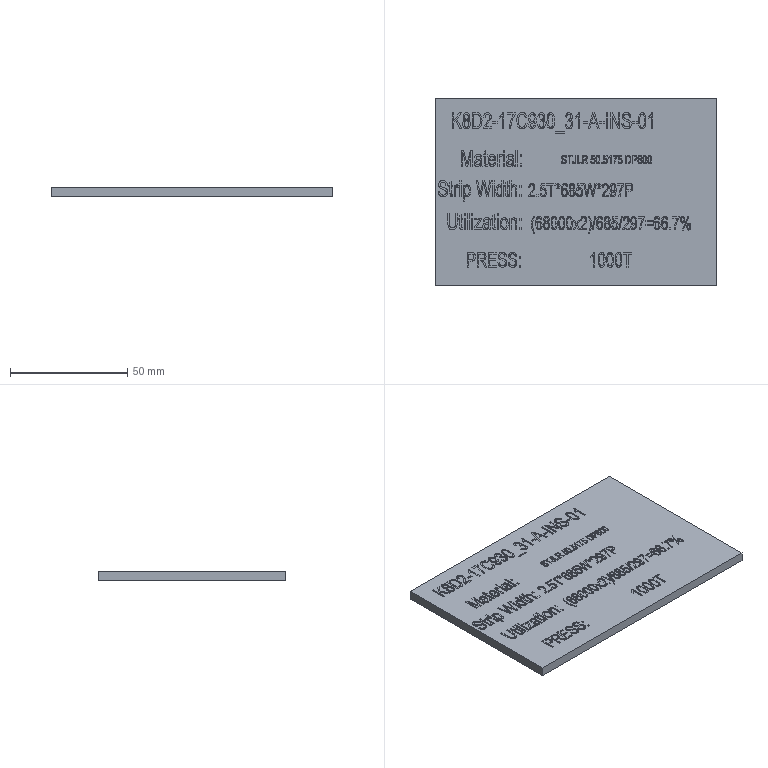Part | STEP file | lll_id1058_x_t | 1 solid | 1575 faces | box 120 x 80 x 4 mm | volume 38260 mm3 | other 833 | plane 742